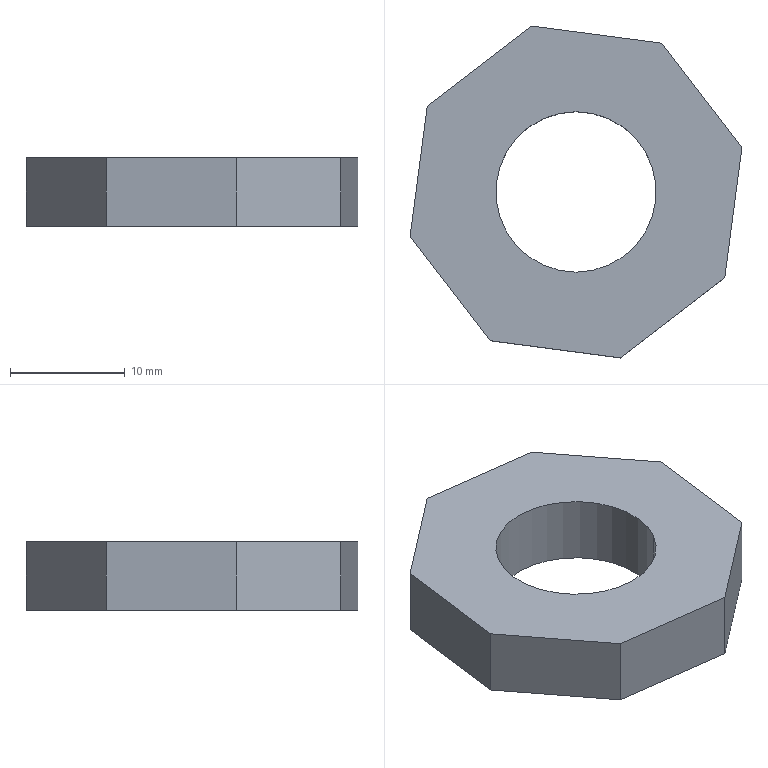Part | SolidWorks | features BaseBody 1 | 1 solid | 12 faces | box 28.978 x 28.978 x 6 mm | volume 2895 mm3 | plane 10 | cylinder 2 | commonest cylinder face diameters 14 x2
STEP:
#1=CARTESIAN_POINT('',(487.224,-33.347,437.));
#2=VERTEX_POINT('',#1);
#3=CARTESIAN_POINT('',(475.1,-26.347,437.));
#4=VERTEX_POINT('',#3);
#5=CARTESIAN_POINT('',(481.162,-29.847,437.));
#6=DIRECTION('',(0.,0.,1.));
#7=DIRECTION('',(-0.866,0.5,0.));
#8=AXIS2_PLACEMENT_3D('',#5,#6,#7);
#9=CIRCLE('',#8,7.);
#10=EDGE_CURVE('',#2,#4,#9,.T.);
#11=ORIENTED_EDGE('',*,*,#10,.T.);
#12=CARTESIAN_POINT('',(475.1,-26.347,431.));
#13=VERTEX_POINT('',#12);
#14=CARTESIAN_POINT('',(475.1,-26.347,437.));
#15=DIRECTION('',(0.,0.,-1.));
#16=VECTOR('',#15,1000.);
#17=LINE('',#14,#16);
#18=EDGE_CURVE('',#4,#13,#17,.T.);
#19=ORIENTED_EDGE('',*,*,#18,.T.);
#20=CARTESIAN_POINT('',(487.224,-33.347,431.));
#21=VERTEX_POINT('',#20);
#22=CARTESIAN_POINT('',(481.162,-29.847,431.));
#23=DIRECTION('',(0.,0.,1.));
#24=DIRECTION('',(-0.866,0.5,0.));
#25=AXIS2_PLACEMENT_3D('',#22,#23,#24);
#26=CIRCLE('',#25,7.);
#27=EDGE_CURVE('',#21,#13,#26,.T.);
#28=ORIENTED_EDGE('',*,*,#27,.F.);
#29=CARTESIAN_POINT('',(487.224,-33.347,437.));
#30=DIRECTION('',(0.,0.,-1.));
#31=VECTOR('',#30,1000.);
#32=LINE('',#29,#31);
#33=EDGE_CURVE('',#2,#21,#32,.T.);
#34=ORIENTED_EDGE('',*,*,#33,.F.);
#35=EDGE_LOOP('',(#11,#19,#28,#34));
#36=FACE_OUTER_BOUND('',#35,.T.);
#37=CARTESIAN_POINT('',(481.162,-29.847,437.));
#38=DIRECTION('',(0.,0.,-1.));
#39=DIRECTION('',(0.866,-0.5,0.));
#40=AXIS2_PLACEMENT_3D('',#37,#38,#39);
#41=CYLINDRICAL_SURFACE('',#40,7.);
#42=ADVANCED_FACE('',(#36),#41,.F.);
#43=CARTESIAN_POINT('',(468.172,-22.347,437.));
#44=VERTEX_POINT('',#43);
#45=CARTESIAN_POINT('',(466.673,-33.729,437.));
#46=VERTEX_POINT('',#45);
#47=CARTESIAN_POINT('',(468.172,-22.347,437.));
#48=DIRECTION('',(-0.1305,-0.9914,0.));
#49=VECTOR('',#48,1000.);
#50=LINE('',#47,#49);
#51=EDGE_CURVE('',#44,#46,#50,.T.);
#52=ORIENTED_EDGE('',*,*,#51,.T.);
#53=CARTESIAN_POINT('',(473.662,-42.837,437.));
#54=VERTEX_POINT('',#53);
#55=CARTESIAN_POINT('',(466.673,-33.729,437.));
#56=DIRECTION('',(0.6088,-0.7934,0.));
#57=VECTOR('',#56,1000.);
#58=LINE('',#55,#57);
#59=EDGE_CURVE('',#46,#54,#58,.T.);
#60=ORIENTED_EDGE('',*,*,#59,.T.);
#61=CARTESIAN_POINT('',(485.044,-44.336,437.));
#62=VERTEX_POINT('',#61);
#63=CARTESIAN_POINT('',(485.044,-44.336,437.));
#64=DIRECTION('',(0.9914,-0.1305,0.));
#65=VECTOR('',#64,1000.);
#66=LINE('',#63,#65);
#67=EDGE_CURVE('',#54,#62,#66,.T.);
#68=ORIENTED_EDGE('',*,*,#67,.T.);
#69=CARTESIAN_POINT('',(494.153,-37.347,437.));
#70=VERTEX_POINT('',#69);
#71=CARTESIAN_POINT('',(494.153,-37.347,437.));
#72=DIRECTION('',(0.7934,0.6088,0.));
#73=VECTOR('',#72,1000.);
#74=LINE('',#71,#73);
#75=EDGE_CURVE('',#62,#70,#74,.T.);
#76=ORIENTED_EDGE('',*,*,#75,.T.);
#77=CARTESIAN_POINT('',(495.651,-25.965,437.));
#78=VERTEX_POINT('',#77);
#79=CARTESIAN_POINT('',(495.651,-25.965,437.));
#80=DIRECTION('',(0.1305,0.9914,0.));
#81=VECTOR('',#80,1000.);
#82=LINE('',#79,#81);
#83=EDGE_CURVE('',#70,#78,#82,.T.);
#84=ORIENTED_EDGE('',*,*,#83,.T.);
#85=CARTESIAN_POINT('',(488.662,-16.856,437.));
#86=VERTEX_POINT('',#85);
#87=CARTESIAN_POINT('',(495.651,-25.965,437.));
#88=DIRECTION('',(-0.6088,0.7934,0.));
#89=VECTOR('',#88,1000.);
#90=LINE('',#87,#89);
#91=EDGE_CURVE('',#78,#86,#90,.T.);
#92=ORIENTED_EDGE('',*,*,#91,.T.);
#93=CARTESIAN_POINT('',(477.28,-15.358,437.));
#94=VERTEX_POINT('',#93);
#95=CARTESIAN_POINT('',(477.28,-15.358,437.));
#96=DIRECTION('',(-0.9914,0.1305,0.));
#97=VECTOR('',#96,1000.);
#98=LINE('',#95,#97);
#99=EDGE_CURVE('',#86,#94,#98,.T.);
#100=ORIENTED_EDGE('',*,*,#99,.T.);
#101=CARTESIAN_POINT('',(477.28,-15.358,437.));
#102=DIRECTION('',(-0.7934,-0.6088,0.));
#103=VECTOR('',#102,1000.);
#104=LINE('',#101,#103);
#105=EDGE_CURVE('',#94,#44,#104,.T.);
#106=ORIENTED_EDGE('',*,*,#105,.T.);
#107=EDGE_LOOP('',(#52,#60,#68,#76,#84,#92,#100,#106));
#108=FACE_OUTER_BOUND('',#107,.T.);
#109=ORIENTED_EDGE('',*,*,#10,.F.);
#110=CARTESIAN_POINT('',(481.162,-29.847,437.));
#111=DIRECTION('',(0.,0.,1.));
#112=DIRECTION('',(-0.866,0.5,0.));
#113=AXIS2_PLACEMENT_3D('',#110,#111,#112);
#114=CIRCLE('',#113,7.);
#115=EDGE_CURVE('',#4,#2,#114,.T.);
#116=ORIENTED_EDGE('',*,*,#115,.F.);
#117=EDGE_LOOP('',(#109,#116));
#118=FACE_BOUND('',#117,.T.);
#119=CARTESIAN_POINT('',(481.162,-29.847,437.));
#120=DIRECTION('',(0.,0.,-1.));
#121=DIRECTION('',(0.866,-0.5,0.));
#122=AXIS2_PLACEMENT_3D('',#119,#120,#121);
#123=PLANE('',#122);
#124=ADVANCED_FACE('',(#108,#118),#123,.F.);
#125=CARTESIAN_POINT('',(468.172,-22.347,431.));
#126=VERTEX_POINT('',#125);
#127=CARTESIAN_POINT('',(466.673,-33.729,431.));
#128=VERTEX_POINT('',#127);
#129=CARTESIAN_POINT('',(468.172,-22.347,431.));
#130=DIRECTION('',(-0.1305,-0.9914,0.));
#131=VECTOR('',#130,1000.);
#132=LINE('',#129,#131);
#133=EDGE_CURVE('',#126,#128,#132,.T.);
#134=ORIENTED_EDGE('',*,*,#133,.F.);
#135=CARTESIAN_POINT('',(477.28,-15.358,431.));
#136=VERTEX_POINT('',#135);
#137=CARTESIAN_POINT('',(477.28,-15.358,431.));
#138=DIRECTION('',(-0.7934,-0.6088,0.));
#139=VECTOR('',#138,1000.);
#140=LINE('',#137,#139);
#141=EDGE_CURVE('',#136,#126,#140,.T.);
#142=ORIENTED_EDGE('',*,*,#141,.F.);
#143=CARTESIAN_POINT('',(488.662,-16.856,431.));
#144=VERTEX_POINT('',#143);
#145=CARTESIAN_POINT('',(477.28,-15.358,431.));
#146=DIRECTION('',(-0.9914,0.1305,0.));
#147=VECTOR('',#146,1000.);
#148=LINE('',#145,#147);
#149=EDGE_CURVE('',#144,#136,#148,.T.);
#150=ORIENTED_EDGE('',*,*,#149,.F.);
#151=CARTESIAN_POINT('',(495.651,-25.965,431.));
#152=VERTEX_POINT('',#151);
#153=CARTESIAN_POINT('',(495.651,-25.965,431.));
#154=DIRECTION('',(-0.6088,0.7934,0.));
#155=VECTOR('',#154,1000.);
#156=LINE('',#153,#155);
#157=EDGE_CURVE('',#152,#144,#156,.T.);
#158=ORIENTED_EDGE('',*,*,#157,.F.);
#159=CARTESIAN_POINT('',(494.153,-37.347,431.));
#160=VERTEX_POINT('',#159);
#161=CARTESIAN_POINT('',(495.651,-25.965,431.));
#162=DIRECTION('',(0.1305,0.9914,0.));
#163=VECTOR('',#162,1000.);
#164=LINE('',#161,#163);
#165=EDGE_CURVE('',#160,#152,#164,.T.);
#166=ORIENTED_EDGE('',*,*,#165,.F.);
#167=CARTESIAN_POINT('',(485.044,-44.336,431.));
#168=VERTEX_POINT('',#167);
#169=CARTESIAN_POINT('',(494.153,-37.347,431.));
#170=DIRECTION('',(0.7934,0.6088,0.));
#171=VECTOR('',#170,1000.);
#172=LINE('',#169,#171);
#173=EDGE_CURVE('',#168,#160,#172,.T.);
#174=ORIENTED_EDGE('',*,*,#173,.F.);
#175=CARTESIAN_POINT('',(473.662,-42.837,431.));
#176=VERTEX_POINT('',#175);
#177=CARTESIAN_POINT('',(485.044,-44.336,431.));
#178=DIRECTION('',(0.9914,-0.1305,0.));
#179=VECTOR('',#178,1000.);
#180=LINE('',#177,#179);
#181=EDGE_CURVE('',#176,#168,#180,.T.);
#182=ORIENTED_EDGE('',*,*,#181,.F.);
#183=CARTESIAN_POINT('',(466.673,-33.729,431.));
#184=DIRECTION('',(0.6088,-0.7934,0.));
#185=VECTOR('',#184,1000.);
#186=LINE('',#183,#185);
#187=EDGE_CURVE('',#128,#176,#186,.T.);
#188=ORIENTED_EDGE('',*,*,#187,.F.);
#189=EDGE_LOOP('',(#134,#142,#150,#158,#166,#174,#182,#188));
#190=FACE_OUTER_BOUND('',#189,.T.);
#191=ORIENTED_EDGE('',*,*,#27,.T.);
#192=CARTESIAN_POINT('',(481.162,-29.847,431.));
#193=DIRECTION('',(0.,0.,1.));
#194=DIRECTION('',(-0.866,0.5,0.));
#195=AXIS2_PLACEMENT_3D('',#192,#193,#194);
#196=CIRCLE('',#195,7.);
#197=EDGE_CURVE('',#13,#21,#196,.T.);
#198=ORIENTED_EDGE('',*,*,#197,.T.);
#199=EDGE_LOOP('',(#191,#198));
#200=FACE_BOUND('',#199,.T.);
#201=CARTESIAN_POINT('',(481.162,-29.847,431.));
#202=DIRECTION('',(0.,0.,-1.));
#203=DIRECTION('',(0.866,-0.5,0.));
#204=AXIS2_PLACEMENT_3D('',#201,#202,#203);
#205=PLANE('',#204);
#206=ADVANCED_FACE('',(#190,#200),#205,.T.);
#207=ORIENTED_EDGE('',*,*,#133,.T.);
#208=CARTESIAN_POINT('',(466.673,-33.729,437.));
#209=DIRECTION('',(0.,0.,-1.));
#210=VECTOR('',#209,1000.);
#211=LINE('',#208,#210);
#212=EDGE_CURVE('',#46,#128,#211,.T.);
#213=ORIENTED_EDGE('',*,*,#212,.F.);
#214=ORIENTED_EDGE('',*,*,#51,.F.);
#215=CARTESIAN_POINT('',(468.172,-22.347,437.));
#216=DIRECTION('',(0.,0.,-1.));
#217=VECTOR('',#216,1000.);
#218=LINE('',#215,#217);
#219=EDGE_CURVE('',#44,#126,#218,.T.);
#220=ORIENTED_EDGE('',*,*,#219,.T.);
#221=EDGE_LOOP('',(#207,#213,#214,#220));
#222=FACE_OUTER_BOUND('',#221,.T.);
#223=CARTESIAN_POINT('',(468.172,-22.347,437.));
#224=DIRECTION('',(0.9914,-0.1305,0.));
#225=DIRECTION('',(0.1305,0.9914,0.));
#226=AXIS2_PLACEMENT_3D('',#223,#224,#225);
#227=PLANE('',#226);
#228=ADVANCED_FACE('',(#222),#227,.F.);
#229=ORIENTED_EDGE('',*,*,#187,.T.);
#230=CARTESIAN_POINT('',(473.662,-42.837,437.));
#231=DIRECTION('',(0.,0.,-1.));
#232=VECTOR('',#231,1000.);
#233=LINE('',#230,#232);
#234=EDGE_CURVE('',#54,#176,#233,.T.);
#235=ORIENTED_EDGE('',*,*,#234,.F.);
#236=ORIENTED_EDGE('',*,*,#59,.F.);
#237=ORIENTED_EDGE('',*,*,#212,.T.);
#238=EDGE_LOOP('',(#229,#235,#236,#237));
#239=FACE_OUTER_BOUND('',#238,.T.);
#240=CARTESIAN_POINT('',(466.673,-33.729,437.));
#241=DIRECTION('',(0.7934,0.6088,0.));
#242=DIRECTION('',(-0.6088,0.7934,0.));
#243=AXIS2_PLACEMENT_3D('',#240,#241,#242);
#244=PLANE('',#243);
#245=ADVANCED_FACE('',(#239),#244,.F.);
#246=ORIENTED_EDGE('',*,*,#181,.T.);
#247=CARTESIAN_POINT('',(485.044,-44.336,437.));
#248=DIRECTION('',(0.,0.,-1.));
#249=VECTOR('',#248,1000.);
#250=LINE('',#247,#249);
#251=EDGE_CURVE('',#62,#168,#250,.T.);
#252=ORIENTED_EDGE('',*,*,#251,.F.);
#253=ORIENTED_EDGE('',*,*,#67,.F.);
#254=ORIENTED_EDGE('',*,*,#234,.T.);
#255=EDGE_LOOP('',(#246,#252,#253,#254));
#256=FACE_OUTER_BOUND('',#255,.T.);
#257=CARTESIAN_POINT('',(485.044,-44.336,437.));
#258=DIRECTION('',(0.1305,0.9914,0.));
#259=DIRECTION('',(-0.9914,0.1305,0.));
#260=AXIS2_PLACEMENT_3D('',#257,#258,#259);
#261=PLANE('',#260);
#262=ADVANCED_FACE('',(#256),#261,.F.);
#263=ORIENTED_EDGE('',*,*,#173,.T.);
#264=CARTESIAN_POINT('',(494.153,-37.347,437.));
#265=DIRECTION('',(0.,0.,-1.));
#266=VECTOR('',#265,1000.);
#267=LINE('',#264,#266);
#268=EDGE_CURVE('',#70,#160,#267,.T.);
#269=ORIENTED_EDGE('',*,*,#268,.F.);
#270=ORIENTED_EDGE('',*,*,#75,.F.);
#271=ORIENTED_EDGE('',*,*,#251,.T.);
#272=EDGE_LOOP('',(#263,#269,#270,#271));
#273=FACE_OUTER_BOUND('',#272,.T.);
#274=CARTESIAN_POINT('',(494.153,-37.347,437.));
#275=DIRECTION('',(-0.6088,0.7934,0.));
#276=DIRECTION('',(-0.7934,-0.6088,0.));
#277=AXIS2_PLACEMENT_3D('',#274,#275,#276);
#278=PLANE('',#277);
#279=ADVANCED_FACE('',(#273),#278,.F.);
#280=ORIENTED_EDGE('',*,*,#165,.T.);
#281=CARTESIAN_POINT('',(495.651,-25.965,437.));
#282=DIRECTION('',(0.,0.,-1.));
#283=VECTOR('',#282,1000.);
#284=LINE('',#281,#283);
#285=EDGE_CURVE('',#78,#152,#284,.T.);
#286=ORIENTED_EDGE('',*,*,#285,.F.);
#287=ORIENTED_EDGE('',*,*,#83,.F.);
#288=ORIENTED_EDGE('',*,*,#268,.T.);
#289=EDGE_LOOP('',(#280,#286,#287,#288));
#290=FACE_OUTER_BOUND('',#289,.T.);
#291=CARTESIAN_POINT('',(495.651,-25.965,437.));
#292=DIRECTION('',(-0.9914,0.1305,0.));
#293=DIRECTION('',(-0.1305,-0.9914,0.));
#294=AXIS2_PLACEMENT_3D('',#291,#292,#293);
#295=PLANE('',#294);
#296=ADVANCED_FACE('',(#290),#295,.F.);
#297=ORIENTED_EDGE('',*,*,#157,.T.);
#298=CARTESIAN_POINT('',(488.662,-16.856,437.));
#299=DIRECTION('',(0.,0.,-1.));
#300=VECTOR('',#299,1000.);
#301=LINE('',#298,#300);
#302=EDGE_CURVE('',#86,#144,#301,.T.);
#303=ORIENTED_EDGE('',*,*,#302,.F.);
#304=ORIENTED_EDGE('',*,*,#91,.F.);
#305=ORIENTED_EDGE('',*,*,#285,.T.);
#306=EDGE_LOOP('',(#297,#303,#304,#305));
#307=FACE_OUTER_BOUND('',#306,.T.);
#308=CARTESIAN_POINT('',(495.651,-25.965,437.));
#309=DIRECTION('',(-0.7934,-0.6088,0.));
#310=DIRECTION('',(0.6088,-0.7934,0.));
#311=AXIS2_PLACEMENT_3D('',#308,#309,#310);
#312=PLANE('',#311);
#313=ADVANCED_FACE('',(#307),#312,.F.);
#314=ORIENTED_EDGE('',*,*,#149,.T.);
#315=CARTESIAN_POINT('',(477.28,-15.358,437.));
#316=DIRECTION('',(0.,0.,-1.));
#317=VECTOR('',#316,1000.);
#318=LINE('',#315,#317);
#319=EDGE_CURVE('',#94,#136,#318,.T.);
#320=ORIENTED_EDGE('',*,*,#319,.F.);
#321=ORIENTED_EDGE('',*,*,#99,.F.);
#322=ORIENTED_EDGE('',*,*,#302,.T.);
#323=EDGE_LOOP('',(#314,#320,#321,#322));
#324=FACE_OUTER_BOUND('',#323,.T.);
#325=CARTESIAN_POINT('',(477.28,-15.358,437.));
#326=DIRECTION('',(-0.1305,-0.9914,0.));
#327=DIRECTION('',(0.9914,-0.1305,0.));
#328=AXIS2_PLACEMENT_3D('',#325,#326,#327);
#329=PLANE('',#328);
#330=ADVANCED_FACE('',(#324),#329,.F.);
#331=ORIENTED_EDGE('',*,*,#141,.T.);
#332=ORIENTED_EDGE('',*,*,#219,.F.);
#333=ORIENTED_EDGE('',*,*,#105,.F.);
#334=ORIENTED_EDGE('',*,*,#319,.T.);
#335=EDGE_LOOP('',(#331,#332,#333,#334));
#336=FACE_OUTER_BOUND('',#335,.T.);
#337=CARTESIAN_POINT('',(477.28,-15.358,437.));
#338=DIRECTION('',(0.6088,-0.7934,0.));
#339=DIRECTION('',(0.7934,0.6088,0.));
#340=AXIS2_PLACEMENT_3D('',#337,#338,#339);
#341=PLANE('',#340);
#342=ADVANCED_FACE('',(#336),#341,.F.);
#343=ORIENTED_EDGE('',*,*,#18,.F.);
#344=ORIENTED_EDGE('',*,*,#115,.T.);
#345=ORIENTED_EDGE('',*,*,#33,.T.);
#346=ORIENTED_EDGE('',*,*,#197,.F.);
#347=EDGE_LOOP('',(#343,#344,#345,#346));
#348=FACE_OUTER_BOUND('',#347,.T.);
#349=CARTESIAN_POINT('',(481.162,-29.847,437.));
#350=DIRECTION('',(0.,0.,-1.));
#351=DIRECTION('',(0.866,-0.5,0.));
#352=AXIS2_PLACEMENT_3D('',#349,#350,#351);
#353=CYLINDRICAL_SURFACE('',#352,7.);
#354=ADVANCED_FACE('',(#348),#353,.F.);
#355=CLOSED_SHELL('',(#42,#124,#206,#228,#245,#262,#279,#296,#313,#330,#342,#354));
#356=MANIFOLD_SOLID_BREP('',#355);
#357=CARTESIAN_POINT('',(0.,0.,0.));
#358=DIRECTION('',(0.,0.,1.));
#359=DIRECTION('',(1.,0.,0.));
#360=AXIS2_PLACEMENT_3D('',#357,#358,#359);
#361=(LENGTH_UNIT()NAMED_UNIT(*)SI_UNIT(.MILLI.,.METRE.));
#362=UNCERTAINTY_MEASURE_WITH_UNIT(LENGTH_MEASURE(0.00001),#361,'','');
#363=(NAMED_UNIT(*)PLANE_ANGLE_UNIT()SI_UNIT($,.RADIAN.));
#364=(NAMED_UNIT(*)SI_UNIT($,.STERADIAN.)SOLID_ANGLE_UNIT());
#365=(GEOMETRIC_REPRESENTATION_CONTEXT(3)GLOBAL_UNCERTAINTY_ASSIGNED_CONTEXT((#362))GLOBAL_UNIT_ASSIGNED_CONTEXT((#361,#363,#364))REPRESENTATION_CONTEXT('',''));
#366=ADVANCED_BREP_SHAPE_REPRESENTATION('',(#356,#360),#365);